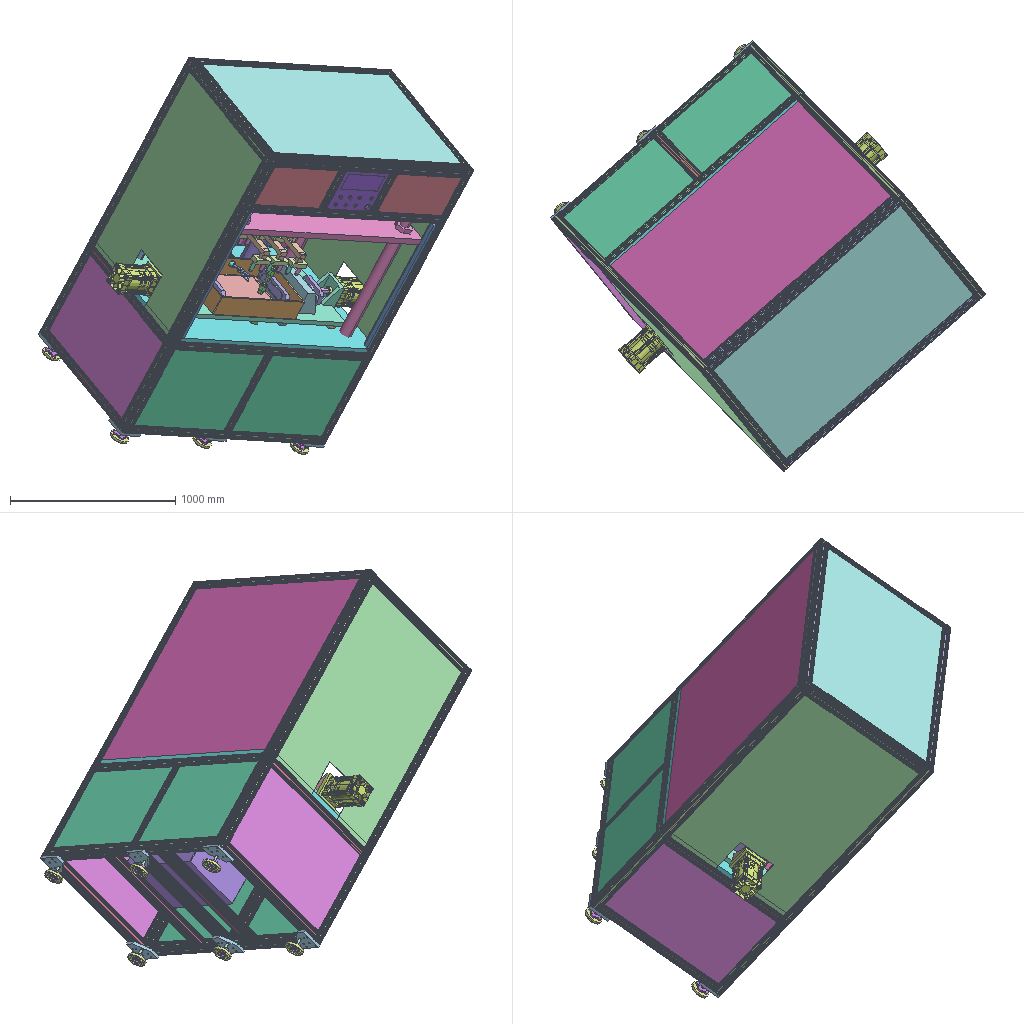Assembly | STEP file | 61 different items | 186 placed | box 2636 x 2611 x 2400 mm
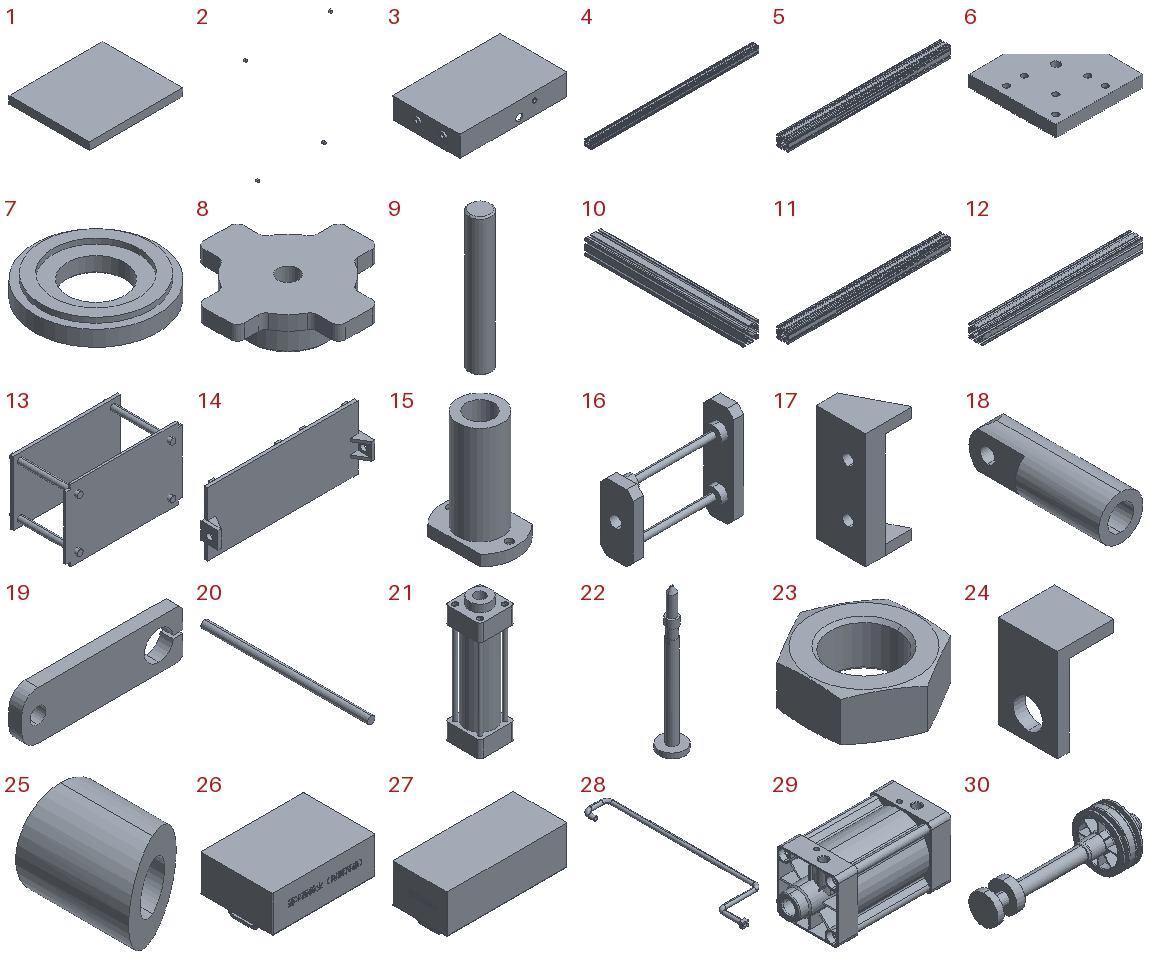Parts list (item | name | quantity | parent item | size | volume):
1 | PN_0008 Pump body base plate | x1 | - | 375 x 320 x 30 mm | 3600000 mm3
2 | Pump body | x1 | - | 260.983 x 5.5 x 336.605 mm | 899.272 mm3
3 | PN_0006 Stainless steel water tank | x1 | - | 694 x 425 x 130 mm | 5429065 mm3
4 | PN_0019 Square aluminium tube_Default <Machined> | x4 | in PN_0023 Small wire lower aluminium alloy frame 5 | 1510 x 60 x 60 mm | 1389788 mm3
5 | PN_0014 Lower outer frame front crossbeam_Default <Machined> | x6 | in PN_0023 Small wire lower aluminium alloy frame 5 | 880 x 60 x 60 mm | 809943 mm3
6 | PN_0022 Foot fixing plate | x6 | in PN_0023 Small wire lower aluminium alloy frame 5 | 150 x 150 x 20 mm | 360114 mm3
7 | Foot | x6 | in Foot sub-assembly | 118 x 118 x 20 mm | 144272 mm3
8 | Foot adjusting disc | x6 | in Foot sub-assembly | 97.968 x 97.968 x 28 mm | 66304 mm3
9 | Foot screw rod | x6 | in Foot sub-assembly | 16 x 16 x 100 mm | 20058 mm3
10 | PN_0025 Lower outer frame column_Default <Machined> | x2 | in PN_0010 Frame support bracket | 60 x 580 x 60 mm | 533826 mm3
11 | PN_0024 Lower outer frame front crossbeam_Default <Machined> | x2 | in PN_0010 Frame support bracket | 880 x 60 x 60 mm | 809943 mm3
12 | PN_0007 Square aluminium tube_Default <Machined> | x4 | in PN_0023 Small wire lower aluminium alloy frame 5 | 700 x 60 x 60 mm | 644273 mm3
13 | PN_0018 Platform plate | x1 | in PN_0023 Small wire lower aluminium alloy frame 5 | 1630 x 960 x 1000 mm | 120961919 mm3
14 | PN_0001 Water tank base plate | x1 | - | 1480 x 180 x 600 mm | 29823409 mm3
15 | Flange linear bearing | x4 | - | 38 x 54 x 80 mm | 46738 mm3
16 | Blocking plate | x2 | - | 341.5 x 100 x 300 mm | 1615392 mm3
17 | PN_0005 Linear bearing seat | x2 | - | 140 x 150 x 350 mm | 3447240 mm3
18 | PN_0021 Connecting shaft | x3 | - | 48 x 150 x 48 mm | 198072 mm3
19 | PN_0015 Guide block | x2 | - | 200 x 16 x 60 mm | 166770 mm3
20 | Plain shaft | x2 | - | 20 x 450 x 20 mm | 141372 mm3
21 | - | x1 | - | 65 x 65 x 237 mm | 394428 mm3
22 | MB50_125_ROD | x1 | - | 50 x 50 x 274.5 mm | 96086 mm3
23 | MB50_NT_05_NUT | x1 | - | 27 x 31.177 x 11 mm | 4552 mm3
24 | PN_0017 Cylinder bracket | x1 | - | 76 x 80 x 126 mm | 217974 mm3
25 | PN_0016 Oil seal | x1 | - | 39 x 49.525 x 39 mm | 35597 mm3
26 | PN_0002 Stainless steel water tank | x1 | - | 600 x 420 x 402 mm | 9376328 mm3
27 | PN_0004 Stainless steel water tank | x1 | - | 820 x 370 x 331.29 mm | 9708465 mm3
28 | Water inlet pipe | x1 | - | 392.5 x 1598 x 50 mm | 595634 mm3
29 | - | x2 | - | 309 x 140 x 140 mm | 1499505 mm3
30 | - | x2 | - | 363 x 124 x 124 mm | 637723 mm3
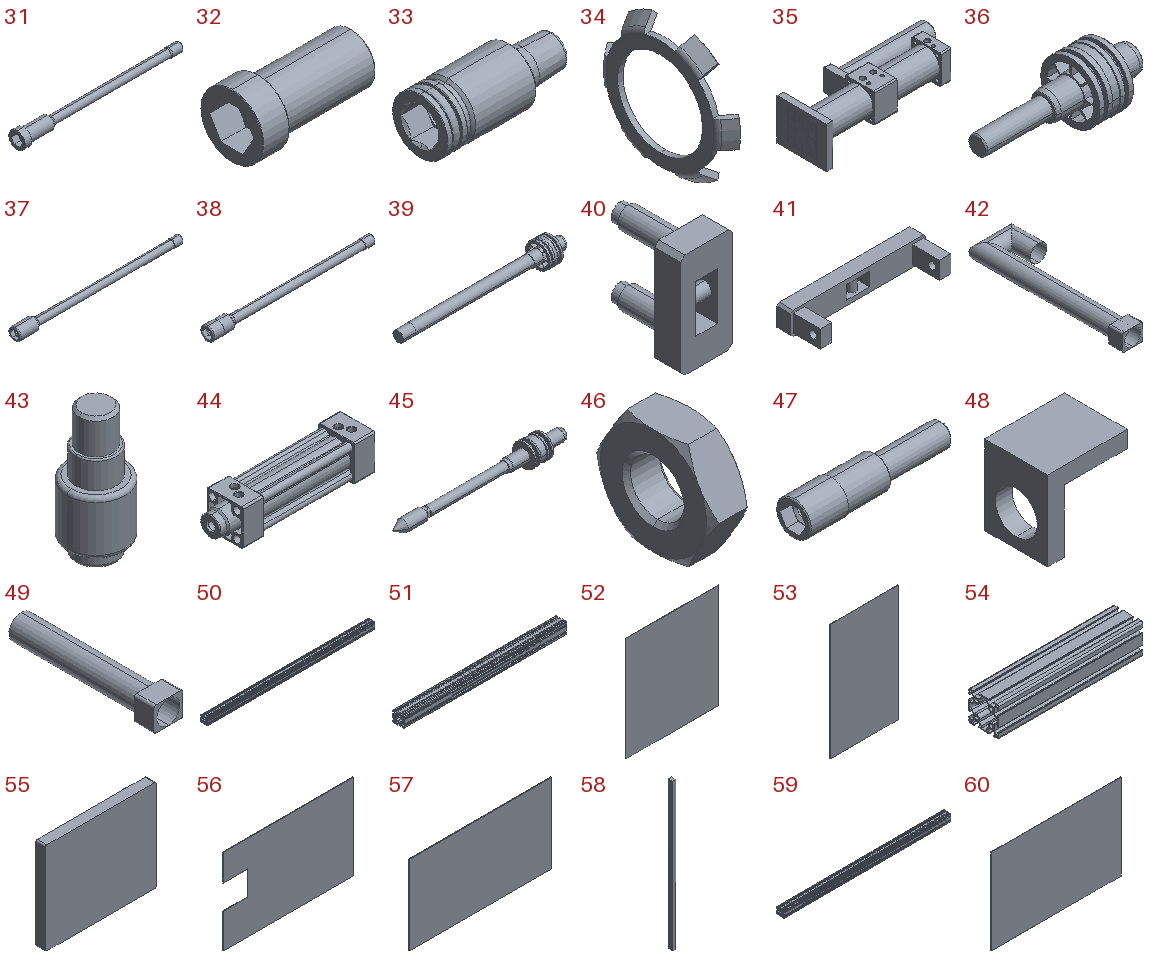31 | SI125_100 | x8 | - | 229 x 23 x 23 mm | 26523 mm3
32 | SI125 | x8 | - | 44 x 23 x 23 mm | 8397 mm3
33 | 125_C_Screw | x4 | - | 24.2 x 10 x 10 mm | 1321 mm3
34 | Outer_ring_gear_1 | x6 | - | 1.224 x 10 x 9.485 mm | 14.03 mm3
35 | SCT_80x100x25_c | x3 | - | 486 x 197 x 132 mm | 2272185 mm3
36 | SCT_80x100x25_r2 | x3 | - | 205 x 79 x 79 mm | 224494 mm3
37 | SCT80_1253 | x12 | - | 214 x 15.5 x 15.5 mm | 15558 mm3
38 | SCT80_1007 | x12 | - | 189 x 15.5 x 15.5 mm | 13853 mm3
39 | SCT_80x100x25_r1 | x3 | - | 553 x 82.1 x 82.1 mm | 687780 mm3
40 | PN_0012 Swing pressure plate | x6 | - | 60 x 100 x 120 mm | 243465 mm3
41 | PN_0003 Connecting bracket | x3 | - | 295 x 90.05 x 50 mm | 507676 mm3
42 | Water outlet pipe 1 | x2 | - | 260 x 905 x 100 mm | 1213100 mm3
43 | Blocking air bag | x2 | - | 43 x 43 x 95 mm | 90813 mm3
44 | - | x1 | - | 196 x 47 x 47 mm | 152031 mm3
45 | - | x1 | - | 235 x 31.5 x 31.5 mm | 41265 mm3
46 | - | x1 | - | 6 x 19.63 x 17 mm | 1126 mm3
47 | SI32_80 | x8 | - | 39 x 9 x 9 mm | 1408 mm3
48 | PN_0009 Cylinder bracket | x1 | - | 76 x 60 x 76 mm | 110454 mm3
49 | Drain pipe 1 | x2 | - | 120 x 605 x 100 mm | 788101 mm3
50 | 1_Default <Machined> | x3 | in PN_0023 Small wire lower aluminium alloy frame 00 | 1510 x 60 x 60 mm | 1389788 mm3
51 | PN_0013 Square aluminium tube_Default <Machined> | x2 | in PN_0023 Small wire lower aluminium alloy frame 00 | 880 x 60 x 60 mm | 809943 mm3
52 | PN_0011 Sealing plate | x1 | in PN_0023 Small wire lower aluminium alloy frame 00 | 1340 x 3 x 1510 mm | 6070200 mm3
53 | PN_0020 Upper sealing plate | x1 | in PN_0023 Small wire lower aluminium alloy frame 00 | 880 x 3 x 1510 mm | 3986400 mm3
54 | Square aluminium tube PN_0026_Default <Machined> | x2 | in PN_0023 Small wire lower aluminium alloy frame 00 | 290 x 60 x 60 mm | 266913 mm3
55 | Part 12 | x1 | in PN_0023 Small wire lower aluminium alloy frame 00 | 350 x 55 x 290 mm | 3054092 mm3
56 | Sealing plate 1 | x2 | in PN_0023 Small wire lower aluminium alloy frame 00 | 1340 x 2 x 880 mm | 2233400 mm3
57 | Sealing plate 4 | x2 | in PN_0023 Small wire lower aluminium alloy frame 00 | 520 x 2 x 290 mm | 301600 mm3
58 | Grating | x2 | in PN_0023 Small wire lower aluminium alloy frame 00 | 20 x 30 x 950 mm | 570000 mm3
59 | 2_Default <Machined> | x4 | in PN_0023 Small wire lower aluminium alloy frame 00 | 1400 x 60 x 60 mm | 1288545 mm3
60 | 880X580 sealing plate | x2 | - | 880 x 2 x 580 mm | 1020800 mm3
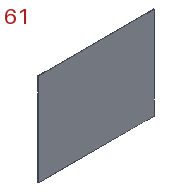61 | 725X580 sealing plate | x4 | - | 725 x 2 x 580 mm | 841000 mm3
Placements (level | parent | child | x y z in mm | rotation matrix by rows):
1 | subassembly 2 | PN_0008 Pump body base plate | 1774.735 96.661 -266.887 | -0.7512 0.5009 0.4299 -0.6586 -0.6125 -0.4371 0.04436 -0.6115 0.79
1 | subassembly 2 | Pump body | 1680.264 104.781 -618.961 | 0.5009 0.4299 -0.7512 -0.6125 -0.4371 -0.6586 -0.6115 0.79 0.04436
1 | subassembly 2 | PN_0006 Stainless steel water tank | 1603.513 -519.23 -362.605 | 0.7512 0.5009 -0.4299 0.6586 -0.6125 0.4371 -0.04436 -0.6115 -0.79
1 | subassembly 2 | PN_0023 Small wire lower aluminium alloy frame 5 | 1076.774 -2632.028 3173.177 | -0.351 0.913 -0.2079 0.5415 0.01685 -0.8405 -0.7639 -0.4076 -0.5003
2 | PN_0023 Small wire lower aluminium alloy frame 5 | PN_0019 Square aluminium tube_Default <Machined> | 4074.198 2232.52 -1426.894 | -0.1268 0.9911 -0.04041 -0.715 -0.06311 0.6963 0.6875 0.1172 0.7166
2 | PN_0023 Small wire lower aluminium alloy frame 5 | PN_0014 Lower outer frame front crossbeam_Default <Machined> | 4711.277 2233.822 -1350.824 | -0.04041 0.1268 -0.9911 0.6963 0.715 0.06311 0.7166 -0.6875 -0.1172
2 | PN_0023 Small wire lower aluminium alloy frame 5 | PN_0019 Square aluminium tube_Default <Machined> | 4708.502 2192.131 -1351.884 | -0.1268 0.9911 -0.04041 -0.715 -0.06311 0.6963 0.6875 0.1172 0.7166
2 | PN_0023 Small wire lower aluminium alloy frame 5 | PN_0022 Foot fixing plate | 4707.221 2908.259 -694.644 | -0.1268 0.04041 0.9911 -0.715 -0.6963 -0.06311 0.6875 -0.7166 0.1172
2 | PN_0023 Small wire lower aluminium alloy frame 5 | PN_0022 Foot fixing plate | 4747.633 2211.988 -1411.284 | -0.04041 -0.1268 0.9911 0.6963 -0.715 -0.06311 0.7166 0.6875 0.1172
2 | PN_0023 Small wire lower aluminium alloy frame 5 | PN_0019 Square aluminium tube_Default <Machined> | 4670.515 2846.626 -678.242 | -0.1268 0.9911 -0.04041 -0.715 -0.06311 0.6963 0.6875 0.1172 0.7166
2 | PN_0023 Small wire lower aluminium alloy frame 5 | PN_0022 Foot fixing plate | 4648.071 1650.714 -871.578 | -0.04041 -0.1268 0.9911 0.6963 -0.715 -0.06311 0.7166 0.6875 0.1172
2 | PN_0023 Small wire lower aluminium alloy frame 5 | PN_0022 Foot fixing plate | 4605.677 2347.11 -155.172 | -0.1268 0.04041 0.9911 -0.715 -0.6963 -0.06311 0.6875 -0.7166 0.1172
2 | PN_0023 Small wire lower aluminium alloy frame 5 | Foot sub-assembly | 4818.807 2204.812 -1274.713 | 0.1148 0.06738 0.9911 -0.04046 0.9972 -0.06311 -0.9926 -0.03286 0.1172
3 | Foot sub-assembly | Foot | -0.0 0.0 -0.0 | 1 0 0 0 1 0 0 0 1
3 | Foot sub-assembly | Foot adjusting disc | -0.0 0.0 13.0 | -0.3643 -0.9313 0 -0.9313 0.3643 0 0 0 -1
3 | Foot sub-assembly | Foot screw rod | -0.0 0.0 -87.0 | 0.8876 -0.4607 0 0.4607 0.8876 0 0 0 1
2 | PN_0023 Small wire lower aluminium alloy frame 5 | Foot sub-assembly | 4719.245 1643.537 -735.006 | 0.1148 0.06738 0.9911 -0.04046 0.9972 -0.06311 -0.9926 -0.03286 0.1172
3 | Foot sub-assembly | Foot | -0.0 0.0 -0.0 | 1 0 0 0 1 0 0 0 1
3 | Foot sub-assembly | Foot adjusting disc | -0.0 0.0 13.0 | -0.3643 -0.9313 0 -0.9313 0.3643 0 0 0 -1
3 | Foot sub-assembly | Foot screw rod | -0.0 0.0 -87.0 | 0.8876 -0.4607 0 0.4607 0.8876 0 0 0 1
2 | PN_0023 Small wire lower aluminium alloy frame 5 | Foot sub-assembly | 4684.125 2214.606 -147.595 | 0.1148 0.06738 0.9911 -0.04046 0.9972 -0.06311 -0.9926 -0.03286 0.1172
3 | Foot sub-assembly | Foot | -0.0 0.0 -0.0 | 1 0 0 0 1 0 0 0 1
3 | Foot sub-assembly | Foot adjusting disc | -0.0 0.0 13.0 | -0.3643 -0.9313 0 -0.9313 0.3643 0 0 0 -1
3 | Foot sub-assembly | Foot screw rod | -0.0 0.0 -87.0 | 0.8876 -0.4607 0 0.4607 0.8876 0 0 0 1
2 | PN_0023 Small wire lower aluminium alloy frame 5 | Foot sub-assembly | 4785.669 2775.754 -687.068 | 0.1148 0.06738 0.9911 -0.04046 0.9972 -0.06311 -0.9926 -0.03286 0.1172
3 | Foot sub-assembly | Foot | -0.0 0.0 -0.0 | 1 0 0 0 1 0 0 0 1
3 | Foot sub-assembly | Foot adjusting disc | -0.0 0.0 13.0 | -0.3643 -0.9313 0 -0.9313 0.3643 0 0 0 -1
3 | Foot sub-assembly | Foot screw rod | -0.0 0.0 -87.0 | 0.8876 -0.4607 0 0.4607 0.8876 0 0 0 1
2 | PN_0023 Small wire lower aluminium alloy frame 5 | PN_0010 Frame support bracket | 4747.75 1909.131 -414.465 | -0.04041 -0.9911 -0.1268 0.6963 0.06311 -0.715 0.7166 -0.1172 0.6875
3 | PN_0010 Frame support bracket | PN_0025 Lower outer frame column_Default <Machined> | -472.918 196.059 -86.541 | 1 0 0 0 1 0 0 0 1
3 | PN_0010 Frame support bracket | PN_0024 Lower outer frame front crossbeam_Default <Machined> | -443.486 165.491 -86.541 | 1 0 0 0 1 0 0 0 1
3 | PN_0010 Frame support bracket | PN_0025 Lower outer frame column_Default <Machined> | 467.082 196.059 -86.541 | 1 0 0 0 1 0 0 0 1
3 | PN_0010 Frame support bracket | PN_0024 Lower outer frame front crossbeam_Default <Machined> | -443.486 805.491 -86.541 | 1 0 0 0 1 0 0 0 1
2 | PN_0023 Small wire lower aluminium alloy frame 5 | Foot sub-assembly | 4634.903 1168.063 -277.803 | 0.1208 0.05598 0.9911 0.05598 0.9964 -0.06311 -0.9911 0.06311 0.1172
3 | Foot sub-assembly | Foot | -0.0 0.0 -0.0 | 1 0 0 0 1 0 0 0 1
3 | Foot sub-assembly | Foot adjusting disc | -0.0 0.0 13.0 | -0.3643 -0.9313 0 -0.9313 0.3643 0 0 0 -1
3 | Foot sub-assembly | Foot screw rod | -0.0 0.0 -87.0 | 0.8876 -0.4607 0 0.4607 0.8876 0 0 0 1
2 | PN_0023 Small wire lower aluminium alloy frame 5 | PN_0022 Foot fixing plate | 4540.9 1046.539 -290.62 | 0.1268 -0.04041 0.9911 0.715 0.6963 -0.06311 -0.6875 0.7166 0.1172
2 | PN_0023 Small wire lower aluminium alloy frame 5 | PN_0022 Foot fixing plate | 4500.488 1742.81 426.021 | 0.04041 0.1268 0.9911 -0.6963 0.715 -0.06311 -0.7166 -0.6875 0.1172
2 | PN_0023 Small wire lower aluminium alloy frame 5 | Foot sub-assembly | 4601.765 1739.005 309.843 | 0.1208 0.05598 0.9911 0.05598 0.9964 -0.06311 -0.9911 0.06311 0.1172
3 | Foot sub-assembly | Foot | -0.0 0.0 -0.0 | 1 0 0 0 1 0 0 0 1
3 | Foot sub-assembly | Foot adjusting disc | -0.0 0.0 13.0 | -0.3643 -0.9313 0 -0.9313 0.3643 0 0 0 -1
3 | Foot sub-assembly | Foot screw rod | -0.0 0.0 -87.0 | 0.8876 -0.4607 0 0.4607 0.8876 0 0 0 1
2 | PN_0023 Small wire lower aluminium alloy frame 5 | PN_0014 Lower outer frame front crossbeam_Default <Machined> | 4512.154 1111.273 -271.411 | -0.04041 0.1268 -0.9911 0.6963 0.715 0.06311 0.7166 -0.6875 -0.1172
2 | PN_0023 Small wire lower aluminium alloy frame 5 | PN_0014 Lower outer frame front crossbeam_Default <Machined> | 4076.972 2274.211 -1425.834 | -0.04041 0.1268 -0.9911 0.6963 0.715 0.06311 0.7166 -0.6875 -0.1172
2 | PN_0023 Small wire lower aluminium alloy frame 5 | PN_0019 Square aluminium tube_Default <Machined> | 4036.21 2887.014 -753.252 | -0.1268 0.9911 -0.04041 -0.715 -0.06311 0.6963 0.6875 0.1172 0.7166
2 | PN_0023 Small wire lower aluminium alloy frame 5 | PN_0007 Square aluminium tube_Default <Machined> | 4048.76 2255.421 -1450.579 | 0.9911 0.1268 -0.04041 -0.06311 0.715 0.6963 0.1172 -0.6875 0.7166
2 | PN_0023 Small wire lower aluminium alloy frame 5 | PN_0007 Square aluminium tube_Default <Machined> | 3849.637 1132.872 -371.166 | 0.9911 0.1268 -0.04041 -0.06311 0.715 0.6963 0.1172 -0.6875 0.7166
2 | PN_0023 Small wire lower aluminium alloy frame 5 | PN_0014 Lower outer frame front crossbeam_Default <Machined> | 3877.849 1151.661 -346.421 | -0.04041 0.1268 -0.9911 0.6963 0.715 0.06311 0.7166 -0.6875 -0.1172
2 | PN_0023 Small wire lower aluminium alloy frame 5 | PN_0018 Platform plate | 4013.45 2952.434 -776.686 | -0.1268 -0.9911 0.04041 -0.715 0.06311 -0.6963 0.6875 -0.1172 -0.7166
2 | PN_0023 Small wire lower aluminium alloy frame 5 | PN_0007 Square aluminium tube_Default <Machined> | 4010.772 2909.916 -776.937 | 0.9911 0.1268 -0.04041 -0.06311 0.715 0.6963 0.1172 -0.6875 0.7166
2 | PN_0023 Small wire lower aluminium alloy frame 5 | PN_0007 Square aluminium tube_Default <Machined> | 3811.649 1787.366 302.476 | 0.9911 0.1268 -0.04041 -0.06311 0.715 0.6963 0.1172 -0.6875 0.7166
2 | PN_0023 Small wire lower aluminium alloy frame 5 | PN_0014 Lower outer frame front crossbeam_Default <Machined> | 4583.491 1513.433 -658.118 | -0.04041 0.1268 -0.9911 0.6963 0.715 0.06311 0.7166 -0.6875 -0.1172
2 | PN_0023 Small wire lower aluminium alloy frame 5 | PN_0014 Lower outer frame front crossbeam_Default <Machined> | 4644.937 1859.835 -991.208 | -0.04041 0.1268 -0.9911 0.6963 0.715 0.06311 0.7166 -0.6875 -0.1172
1 | subassembly 2 | PN_0001 Water tank base plate | 1284.712 -708.687 -458.509 | 0.7512 -0.4299 -0.5009 0.6586 0.4371 0.6125 -0.04436 -0.79 0.6115
1 | subassembly 2 | Flange linear bearing | 1399.666 -485.661 -317.91 | 0.4299 0.5009 0.7512 -0.4371 -0.6125 0.6586 0.79 -0.6115 -0.04436
1 | subassembly 2 | Flange linear bearing | 1310.923 -378.918 -235.869 | -0.4299 -0.5009 0.7512 0.4371 0.6125 0.6586 -0.79 0.6115 -0.04436
1 | subassembly 2 | Blocking plate | 1267.963 -465.712 -314.948 | 0.7512 0.4299 0.5009 0.6586 -0.4371 -0.6125 -0.04436 0.79 -0.6115
1 | subassembly 2 | PN_0005 Linear bearing seat | 1361.054 -384.094 -320.445 | -0.7512 0.4299 -0.5009 -0.6586 -0.4371 0.6125 0.04436 0.79 0.6115
1 | subassembly 2 | PN_0021 Connecting shaft | 1854.936 -450.673 88.657 | 0.7512 -0.4299 -0.5009 0.6586 0.4371 0.6125 -0.04436 -0.79 0.6115
1 | subassembly 2 | PN_0015 Guide block | 1831.91 -420.038 153.582 | 0.5009 -0.4299 0.7512 -0.6125 0.4371 0.6586 -0.6115 -0.79 -0.04436
1 | subassembly 2 | Plain shaft | 1976.267 -558.568 541.411 | 0.273 -0.4299 0.8606 -0.7711 0.4371 0.4629 -0.5752 -0.79 -0.2122
1 | subassembly 2 | subassembly 3 | 1612.926 -4.684 -130.227 | -0.7929 -0.4299 -0.4318 0.2357 0.4371 -0.868 0.5619 -0.79 -0.2453
2 | subassembly 3 | subassembly 4 | -0.0 -0.0 -0.0 | 0 0 -1 0 1 0 1 0 0
2 | subassembly 3 | MB50_125_ROD | -93.121 -0.0 0.0 | 0 0 -1 0 1 0 1 0 0
2 | subassembly 3 | MB50_NT_05_NUT | -130.621 0.0 0.0 | 0 0 -1 0 1 0 1 0 0
1 | subassembly 2 | PN_0017 Cylinder bracket | 1609.969 -53.959 -113.731 | -0.7929 0.4318 -0.4299 0.2357 0.868 0.4371 0.5619 0.2453 -0.79
1 | subassembly 2 | PN_0016 Oil seal | 1633.542 -10.812 -144.837 | 0.4809 0.7929 -0.3742 0.8084 -0.2357 0.5394 0.3395 -0.5619 -0.7543
1 | subassembly 2 | PN_0002 Stainless steel water tank | 1550.286 554.551 -549.609 | -0.7512 -0.5009 -0.4299 -0.6586 0.6125 0.4371 0.04436 0.6115 -0.79
1 | subassembly 2 | PN_0004 Stainless steel water tank | 2164.955 29.627 749.495 | -0.7512 -0.5009 -0.4299 -0.6586 0.6125 0.4371 0.04436 0.6115 -0.79
1 | subassembly 2 | Water inlet pipe | 1179.037 161.504 -562.536 | -0.7512 0.4299 -0.5009 -0.6586 -0.4371 0.6125 0.04436 0.79 0.6115
1 | subassembly 2 | subassembly 5 | 1162.24 -601.55 -265.49 | -0.7512 0.4299 -0.5009 -0.6586 -0.4371 0.6125 0.04436 0.79 0.6115
2 | subassembly 5 | subassembly 6 | -0.0 -0.0 -0.0 | 1 0 0 0 1 0 0 0 1
2 | subassembly 5 | subassembly 7 | -82.074 -0.0 0.0 | 1 0 0 0 0.7071 0.7071 0 -0.7071 0.7071
2 | subassembly 5 | SI125_100 | 46.0 -55.0 55.0 | 1 0 0 0 1 0 0 0 1
2 | subassembly 5 | SI125_100 | 46.0 -55.0 -55.0 | 1 0 0 0 1 0 0 0 1
2 | subassembly 5 | SI125_100 | 46.0 55.0 55.0 | 1 0 0 0 1 0 0 0 1
2 | subassembly 5 | SI125_100 | 46.0 55.0 -55.0 | 1 0 0 0 1 0 0 0 1
2 | subassembly 5 | SI125 | 214.0 -55.0 55.0 | -1 0 0 0 -1 0 0 0 1
2 | subassembly 5 | SI125 | 214.0 -55.0 -55.0 | -1 0 0 0 -1 0 0 0 1
2 | subassembly 5 | SI125 | 214.0 55.0 55.0 | -1 0 0 0 -1 0 0 0 1
2 | subassembly 5 | SI125 | 214.0 55.0 -55.0 | -1 0 0 0 -1 0 0 0 1
2 | subassembly 5 | 125_C_Screw | 35.0 14.0 66.5 | 0 0 -1 0 -1 0 -1 0 0
2 | subassembly 5 | 125_C_Screw | 225.0 14.0 66.5 | 0 0 -1 0 -1 0 -1 0 0
2 | subassembly 5 | Outer_ring_gear_1 | 35.0 14.0 68.7 | 0 -1 0 0 0 -1 1 0 0
2 | subassembly 5 | Outer_ring_gear_1 | 225.0 14.0 68.7 | 0 -1 0 0 0 -1 1 0 0
1 | subassembly 2 | subassembly 8 | 1929.045 -526.028 224.84 | 0.4299 -0.5009 -0.7512 -0.4371 0.6125 -0.6586 0.79 0.6115 0.04436
2 | subassembly 8 | SCT_80x100x25_c | -0.0 -0.0 -0.0 | 1 0 0 0 1 0 0 0 1
2 | subassembly 8 | SCT_80x100x25_r2 | -0.0 -0.0 -0.0 | 1 0 0 0 1 0 0 0 1
2 | subassembly 8 | SCT80_1253 | 33.0 -35.0 35.0 | 1 0 0 0 1 0 0 0 1
2 | subassembly 8 | SCT80_1253 | 33.0 -35.0 -35.0 | 1 0 0 0 1 0 0 0 1
2 | subassembly 8 | SCT80_1253 | 33.0 35.0 35.0 | 1 0 0 0 1 0 0 0 1
2 | subassembly 8 | SCT80_1253 | 33.0 35.0 -35.0 | 1 0 0 0 1 0 0 0 1
2 | subassembly 8 | SCT80_1007 | 421.5 -35.0 35.0 | -1 0 0 0 -1 0 0 0 1
2 | subassembly 8 | SCT80_1007 | 421.5 -35.0 -35.0 | -1 0 0 0 -1 0 0 0 1
2 | subassembly 8 | SCT80_1007 | 421.5 35.0 35.0 | -1 0 0 0 -1 0 0 0 1
2 | subassembly 8 | SCT80_1007 | 421.5 35.0 -35.0 | -1 0 0 0 -1 0 0 0 1
2 | subassembly 8 | SCT_80x100x25_r1 | 101.616 -1.374 -0.7166 | 1 0 0 0 -0.8867 0.4623 0 -0.4623 -0.8867
1 | subassembly 2 | subassembly 5 | 2273.794 373.382 -331.5 | 0.7512 -0.4299 -0.5009 0.6586 0.4371 0.6125 -0.04436 -0.79 0.6115
2 | subassembly 5 | subassembly 6 | -0.0 -0.0 -0.0 | 1 0 0 0 1 0 0 0 1
2 | subassembly 5 | subassembly 7 | -82.074 -0.0 -0.0 | 1 0 0 0 0.7071 0.7071 0 -0.7071 0.7071
2 | subassembly 5 | SI125_100 | 46.0 -55.0 55.0 | 1 0 0 0 1 0 0 0 1
2 | subassembly 5 | SI125_100 | 46.0 -55.0 -55.0 | 1 0 0 0 1 0 0 0 1
2 | subassembly 5 | SI125_100 | 46.0 55.0 55.0 | 1 0 0 0 1 0 0 0 1
2 | subassembly 5 | SI125_100 | 46.0 55.0 -55.0 | 1 0 0 0 1 0 0 0 1
2 | subassembly 5 | SI125 | 214.0 -55.0 55.0 | -1 0 0 0 -1 0 0 0 1
2 | subassembly 5 | SI125 | 214.0 -55.0 -55.0 | -1 0 0 0 -1 0 0 0 1
2 | subassembly 5 | SI125 | 214.0 55.0 55.0 | -1 0 0 0 -1 0 0 0 1
2 | subassembly 5 | SI125 | 214.0 55.0 -55.0 | -1 0 0 0 -1 0 0 0 1
2 | subassembly 5 | 125_C_Screw | 35.0 14.0 66.5 | 0 0 -1 0 -1 0 -1 0 0
2 | subassembly 5 | 125_C_Screw | 225.0 14.0 66.5 | 0 0 -1 0 -1 0 -1 0 0
2 | subassembly 5 | Outer_ring_gear_1 | 35.0 14.0 68.7 | 0 -1 0 0 0 -1 1 0 0
2 | subassembly 5 | Outer_ring_gear_1 | 225.0 14.0 68.7 | 0 -1 0 0 0 -1 1 0 0
1 | subassembly 2 | PN_0005 Linear bearing seat | 1992.048 169.131 -357.704 | 0.7512 0.4299 0.5009 0.6586 -0.4371 -0.6125 -0.04436 0.79 -0.6115
1 | subassembly 2 | Flange linear bearing | 2079.152 126.361 -374.34 | -0.4299 0.5009 -0.7512 0.4371 -0.6125 -0.6586 -0.79 -0.6115 0.04436
1 | subassembly 2 | Flange linear bearing | 1999.007 224.362 -276.5 | -0.4299 0.5009 -0.7512 0.4371 -0.6125 -0.6586 -0.79 -0.6115 0.04436
1 | subassembly 2 | Blocking plate | 2122.699 283.679 -365.419 | -0.7512 0.4299 -0.5009 -0.6586 -0.4371 0.6125 0.04436 0.79 0.6115
1 | subassembly 2 | PN_0012 Swing pressure plate | 1655.668 -315.469 51.655 | 0.5009 -0.4299 0.7512 -0.6125 0.4371 0.6586 -0.6115 -0.79 -0.04436
1 | subassembly 2 | PN_0012 Swing pressure plate | 1785.903 -474.72 -107.336 | 0.5009 -0.4299 0.7512 -0.6125 0.4371 0.6586 -0.6115 -0.79 -0.04436
1 | subassembly 2 | PN_0003 Connecting bracket | 1738.247 -279.821 63.151 | 0.5009 0.4299 -0.7512 -0.6125 -0.4371 -0.6586 -0.6115 0.79 0.04436
1 | subassembly 2 | PN_0021 Connecting shaft | 2074.543 -272.39 67.8 | 0.7512 -0.4299 -0.5009 0.6586 0.4371 0.6125 -0.04436 -0.79 0.6115
1 | subassembly 2 | PN_0015 Guide block | 2046.359 -236.509 123.245 | 0.5009 -0.4299 0.7512 -0.6125 0.4371 0.6586 -0.6115 -0.79 -0.04436
1 | subassembly 2 | Plain shaft | 2192.865 -377.224 515.024 | 0.718 -0.4299 -0.5474 0.696 0.4371 0.5697 -0.005638 -0.79 0.6131
1 | subassembly 2 | PN_0003 Connecting bracket | 1956.352 -102.855 42.382 | 0.5009 0.4299 -0.7512 -0.6125 -0.4371 -0.6586 -0.6115 0.79 0.04436
1 | subassembly 2 | PN_0012 Swing pressure plate | 2004.008 -297.754 -128.104 | 0.5009 -0.4299 0.7512 -0.6125 0.4371 0.6586 -0.6115 -0.79 -0.04436
1 | subassembly 2 | PN_0012 Swing pressure plate | 1873.773 -138.503 30.887 | 0.5009 -0.4299 0.7512 -0.6125 0.4371 0.6586 -0.6115 -0.79 -0.04436
1 | subassembly 2 | subassembly 8 | 2148.652 -347.745 203.983 | 0.4299 -0.5009 -0.7512 -0.4371 0.6125 -0.6586 0.79 0.6115 0.04436
2 | subassembly 8 | SCT_80x100x25_c | -0.0 -0.0 -0.0 | 1 0 0 0 1 0 0 0 1
2 | subassembly 8 | SCT_80x100x25_r2 | -0.0 -0.0 -0.0 | 1 0 0 0 1 0 0 0 1
2 | subassembly 8 | SCT80_1253 | 33.0 -35.0 35.0 | 1 0 0 0 1 0 0 0 1
2 | subassembly 8 | SCT80_1253 | 33.0 -35.0 -35.0 | 1 0 0 0 1 0 0 0 1
2 | subassembly 8 | SCT80_1253 | 33.0 35.0 35.0 | 1 0 0 0 1 0 0 0 1
2 | subassembly 8 | SCT80_1253 | 33.0 35.0 -35.0 | 1 0 0 0 1 0 0 0 1
2 | subassembly 8 | SCT80_1007 | 421.5 -35.0 35.0 | -1 0 0 0 -1 0 0 0 1
2 | subassembly 8 | SCT80_1007 | 421.5 -35.0 -35.0 | -1 0 0 0 -1 0 0 0 1
2 | subassembly 8 | SCT80_1007 | 421.5 35.0 35.0 | -1 0 0 0 -1 0 0 0 1
2 | subassembly 8 | SCT80_1007 | 421.5 35.0 -35.0 | -1 0 0 0 -1 0 0 0 1
2 | subassembly 8 | SCT_80x100x25_r1 | 101.616 0.1162 1.546 | 1 0 0 0 0.07497 -0.9972 0 0.9972 0.07497
1 | subassembly 2 | Water outlet pipe 1 | 1582.368 -426.242 434.534 | 0.5009 -0.4299 0.7512 -0.6125 0.4371 0.6586 -0.6115 -0.79 -0.04436
1 | subassembly 2 | Blocking air bag | 1861.813 -79.82 -285.345 | 0.1199 0.8949 -0.4299 0.8949 0.09008 0.4371 0.4299 -0.4371 -0.79
1 | subassembly 2 | subassembly 9 | 1691.797 79.824 -185.5 | -0.5009 -0.7512 0.4299 0.6125 -0.6586 -0.4371 0.6115 0.04436 0.79
2 | subassembly 9 | subassembly 10 | -0.0 -0.0 -0.0 | 1 0 0 0 1 0 0 0 1
2 | subassembly 9 | subassembly 11 | -70.589 0.0 -0.0 | 1 0 0 0 0.7071 0.7071 0 -0.7071 0.7071
2 | subassembly 9 | subassembly 12 | 58.561 -0.0 0.0 | 1 0 0 0 -1 0 0 0 -1
2 | subassembly 9 | SI32_80 | 22.5 -16.25 16.25 | 1 0 0 0 1 0 0 0 1
2 | subassembly 9 | SI32_80 | 22.5 -16.25 -16.25 | 1 0 0 0 1 0 0 0 1
2 | subassembly 9 | SI32_80 | 22.5 16.25 16.25 | 1 0 0 0 1 0 0 0 1
2 | subassembly 9 | SI32_80 | 22.5 16.25 -16.25 | 1 0 0 0 1 0 0 0 1
2 | subassembly 9 | SI32_80 | 151.5 -16.25 16.25 | -1 0 0 0 -1 0 0 0 1
2 | subassembly 9 | SI32_80 | 151.5 -16.25 -16.25 | -1 0 0 0 -1 0 0 0 1
2 | subassembly 9 | SI32_80 | 151.5 16.25 16.25 | -1 0 0 0 -1 0 0 0 1
2 | subassembly 9 | SI32_80 | 151.5 16.25 -16.25 | -1 0 0 0 -1 0 0 0 1
2 | subassembly 9 | Outer_ring_gear_1 | 19.0 6.0 22.2 | 0 -1 0 0 0 -1 1 0 -0
2 | subassembly 9 | Outer_ring_gear_1 | 155.0 6.0 22.2 | 0 -1 0 0 0 -1 1 0 -0
1 | subassembly 2 | PN_0009 Cylinder bracket | 1682.159 46.952 -160.47 | -0.5009 0.7512 -0.4299 0.6125 0.6586 0.4371 0.6115 -0.04436 -0.79
1 | subassembly 2 | Water outlet pipe 1 | 1969.227 -87.062 411.691 | 0.5009 -0.4299 0.7512 -0.6125 0.4371 0.6586 -0.6115 -0.79 -0.04436
1 | subassembly 2 | Drain pipe 1 | 1520.883 -294.171 -345.006 | 0.7512 -0.4299 -0.5009 0.6586 0.4371 0.6125 -0.04436 -0.79 0.6115
1 | subassembly 2 | Drain pipe 1 | 1802.244 -47.487 -361.62 | 0.7512 -0.4299 -0.5009 0.6586 0.4371 0.6125 -0.04436 -0.79 0.6115
1 | subassembly 2 | PN_0023 Small wire lower aluminium alloy frame 00 | 11245.612 8377.661 4750.419 | -0.5011 -0.8587 0.1071 0.325 -0.07202 0.943 -0.8021 0.5073 0.3151
2 | PN_0023 Small wire lower aluminium alloy frame 00 | 1_Default <Machined> | 4906.287 7191.602 -10870.07 | -0.1268 0.9911 -0.04041 -0.715 -0.06311 0.6963 0.6875 0.1172 0.7166
2 | PN_0023 Small wire lower aluminium alloy frame 00 | 1_Default <Machined> | 4944.021 6535.677 -11542.337 | -0.1268 0.9911 -0.04041 -0.715 -0.06311 0.6963 0.6875 0.1172 0.7166
2 | PN_0023 Small wire lower aluminium alloy frame 00 | PN_0013 Square aluminium tube_Default <Machined> | 4911.875 7190.046 -10910.558 | 0.04041 0.1268 0.9911 -0.6963 0.715 -0.06311 -0.7166 -0.6875 0.1172
2 | PN_0023 Small wire lower aluminium alloy frame 00 | PN_0013 Square aluminium tube_Default <Machined> | 4712.752 6067.497 -9831.144 | 0.04041 0.1268 0.9911 -0.6963 0.715 -0.06311 -0.7166 -0.6875 0.1172
2 | PN_0023 Small wire lower aluminium alloy frame 00 | PN_0011 Sealing plate | 4935.504 7208.246 -10847.37 | 0.9911 -0.04041 -0.1268 -0.06311 0.6963 -0.715 0.1172 0.7166 0.6875
2 | PN_0023 Small wire lower aluminium alloy frame 00 | PN_0020 Upper sealing plate | 4913.651 6558.197 -11524.52 | -0.04041 -0.9911 -0.1268 0.6963 0.06311 -0.715 0.7166 -0.1172 0.6875
2 | PN_0023 Small wire lower aluminium alloy frame 00 | Square aluminium tube PN_0026_Default <Machined> | 4904.554 6139.646 -11161.032 | 0.9911 -0.04041 -0.1268 -0.06311 0.6963 -0.715 0.1172 0.7166 0.6875
2 | PN_0023 Small wire lower aluminium alloy frame 00 | Part 12 | 4900.768 6118.823 -11140.223 | -0.1268 0.04041 0.9911 -0.715 -0.6963 -0.06311 0.6875 -0.7166 0.1172
2 | PN_0023 Small wire lower aluminium alloy frame 00 | Sealing plate 1 | 6273.239 7125.466 -10771.043 | -0.9911 0.1268 0.04041 0.06311 0.715 -0.6963 -0.1172 -0.6875 -0.7166
2 | PN_0023 Small wire lower aluminium alloy frame 00 | Sealing plate 4 | 4909.59 6140.835 -11202.973 | 0.1268 -0.04041 0.9911 0.715 0.6963 -0.06311 -0.6875 0.7166 0.1172
2 | PN_0023 Small wire lower aluminium alloy frame 00 | Grating | 5327.112 6511.06 -11497.268 | -0.1268 -0.04041 -0.9911 -0.715 0.6963 0.06311 0.6875 0.7166 -0.1172
2 | PN_0023 Small wire lower aluminium alloy frame 00 | Grating | 5146.574 5409.9 -10479.451 | 0.1268 0.04041 -0.9911 0.715 -0.6963 0.06311 -0.6875 -0.7166 -0.1172
2 | PN_0023 Small wire lower aluminium alloy frame 00 | 2_Default <Machined> | 4681.726 6091.954 -9814.342 | 0.9911 0.1268 -0.04041 -0.06311 0.715 0.6963 0.1172 -0.6875 0.7166
2 | PN_0023 Small wire lower aluminium alloy frame 00 | 2_Default <Machined> | 4719.46 5436.03 -10486.609 | 0.9911 0.1268 -0.04041 -0.06311 0.715 0.6963 0.1172 -0.6875 0.7166
2 | PN_0023 Small wire lower aluminium alloy frame 00 | 2_Default <Machined> | 4918.583 6558.579 -11566.022 | 0.9911 0.1268 -0.04041 -0.06311 0.715 0.6963 0.1172 -0.6875 0.7166
2 | PN_0023 Small wire lower aluminium alloy frame 00 | 2_Default <Machined> | 4880.849 7214.504 -10893.755 | 0.9911 0.1268 -0.04041 -0.06311 0.715 0.6963 0.1172 -0.6875 0.7166
2 | PN_0023 Small wire lower aluminium alloy frame 00 | 1_Default <Machined> | 5290.906 6513.59 -11501.316 | -0.1268 0.9911 -0.04041 -0.715 -0.06311 0.6963 0.6875 0.1172 0.7166
2 | PN_0023 Small wire lower aluminium alloy frame 00 | Sealing plate 1 | 6066.506 5960.016 -9650.379 | -0.9911 0.1268 0.04041 0.06311 0.715 -0.6963 -0.1172 -0.6875 -0.7166
2 | PN_0023 Small wire lower aluminium alloy frame 00 | Square aluminium tube PN_0026_Default <Machined> | 4852.554 5846.496 -10879.147 | 0.9911 -0.04041 -0.1268 -0.06311 0.6963 -0.715 0.1172 0.7166 0.6875
2 | PN_0023 Small wire lower aluminium alloy frame 00 | Sealing plate 4 | 4784.028 5432.985 -10522.324 | 0.1268 -0.04041 0.9911 0.715 0.6963 -0.06311 -0.6875 0.7166 0.1172
1 | subassembly 2 | 880X580 sealing plate | 554.431 25.91 -566.018 | 0.5009 0.7512 0.4299 -0.6125 0.6586 -0.4371 -0.6115 -0.04436 0.79
1 | subassembly 2 | 725X580 sealing plate | 1070.352 -510.326 -1143.493 | 0.7512 -0.5009 0.4299 0.6586 0.6125 -0.4371 -0.04436 0.6115 0.79
1 | subassembly 2 | 725X580 sealing plate | 1660.031 6.676 -1178.312 | 0.7512 -0.5009 0.4299 0.6586 0.6125 -0.4371 -0.04436 0.6115 0.79
1 | subassembly 2 | 725X580 sealing plate | 1160.129 617.953 -568.032 | 0.7512 -0.5009 0.4299 0.6586 0.6125 -0.4371 -0.04436 0.6115 0.79
1 | subassembly 2 | 725X580 sealing plate | 570.45 100.951 -533.212 | 0.7512 -0.5009 0.4299 0.6586 0.6125 -0.4371 -0.04436 0.6115 0.79
1 | subassembly 2 | 880X580 sealing plate | 1777.358 1098.113 -638.23 | 0.5009 0.7512 0.4299 -0.6125 0.6586 -0.4371 -0.6115 -0.04436 0.79
1 | subassembly 2 | subassembly 8 | 2034.211 -433.824 218.63 | 0.4299 -0.5009 -0.7512 -0.4371 0.6125 -0.6586 0.79 0.6115 0.04436
2 | subassembly 8 | SCT_80x100x25_c | -0.0 -0.0 -0.0 | 1 0 0 0 1 0 0 0 1
2 | subassembly 8 | SCT_80x100x25_r2 | -0.0 -0.0 -0.0 | 1 0 0 0 1 0 0 0 1
2 | subassembly 8 | SCT80_1253 | 33.0 -35.0 35.0 | 1 0 0 0 1 0 0 0 1
2 | subassembly 8 | SCT80_1253 | 33.0 -35.0 -35.0 | 1 0 0 0 1 0 0 0 1
2 | subassembly 8 | SCT80_1253 | 33.0 35.0 35.0 | 1 0 0 0 1 0 0 0 1
2 | subassembly 8 | SCT80_1253 | 33.0 35.0 -35.0 | 1 0 0 0 1 0 0 0 1
2 | subassembly 8 | SCT80_1007 | 421.5 -35.0 35.0 | -1 0 0 0 -1 0 0 0 1
2 | subassembly 8 | SCT80_1007 | 421.5 -35.0 -35.0 | -1 0 0 0 -1 0 0 0 1
2 | subassembly 8 | SCT80_1007 | 421.5 35.0 35.0 | -1 0 0 0 -1 0 0 0 1
2 | subassembly 8 | SCT80_1007 | 421.5 35.0 -35.0 | -1 0 0 0 -1 0 0 0 1
2 | subassembly 8 | SCT_80x100x25_r1 | -27.547 1.383 -0.6999 | 1 0 0 0 0.8923 0.4515 0 -0.4515 0.8923
1 | subassembly 2 | PN_0021 Connecting shaft | 1960.102 -358.469 82.447 | 0.7512 -0.4299 -0.5009 0.6586 0.4371 0.6125 -0.04436 -0.79 0.6115
1 | subassembly 2 | PN_0003 Connecting bracket | 1841.91 -188.934 57.029 | 0.5009 0.4299 -0.7512 -0.6125 -0.4371 -0.6586 -0.6115 0.79 0.04436
1 | subassembly 2 | PN_0012 Swing pressure plate | 1889.566 -383.833 -113.457 | 0.5009 -0.4299 0.7512 -0.6125 0.4371 0.6586 -0.6115 -0.79 -0.04436
1 | subassembly 2 | PN_0012 Swing pressure plate | 1879.527 -182.3 3.521 | -0.5009 -0.4299 -0.7512 0.6125 0.4371 -0.6586 0.6115 -0.79 0.04436
1 | subassembly 2 | Blocking air bag | 1913.402 -132.276 -190.545 | 0.1199 0.8949 -0.4299 0.8949 0.09008 0.4371 0.4299 -0.4371 -0.79